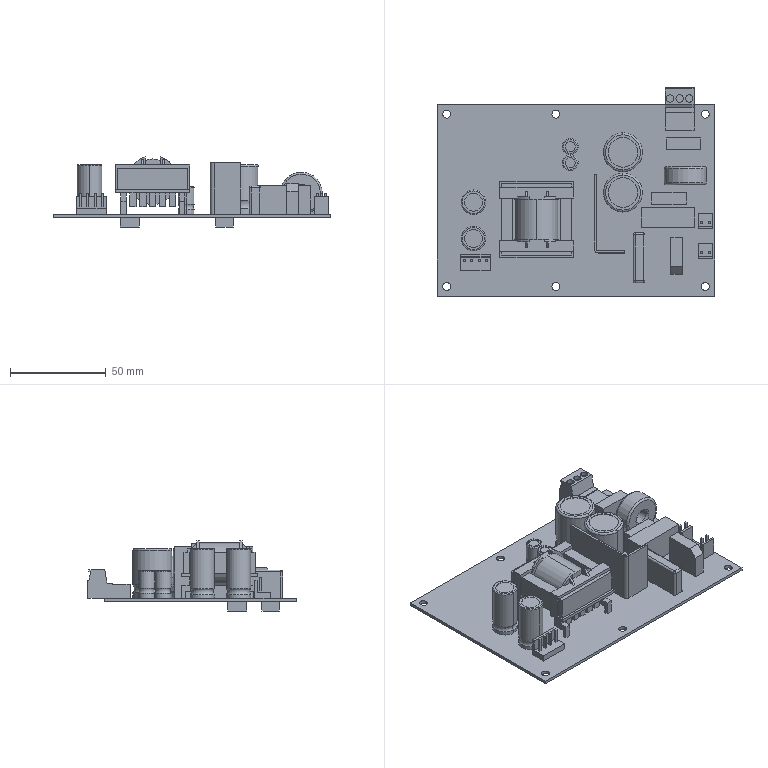Part | STEP file | LIB_64668064 | 2 solids | 423 faces | box 145 x 108.65 x 36.554 mm | volume 90051 mm3 | plane 311 | cylinder 76 | torus 32 | sphere 4 | commonest cylinder face diameters 4.15 x12 2 x8 8.2 x8 12.7 x8 20.3 x8 3.9 x6